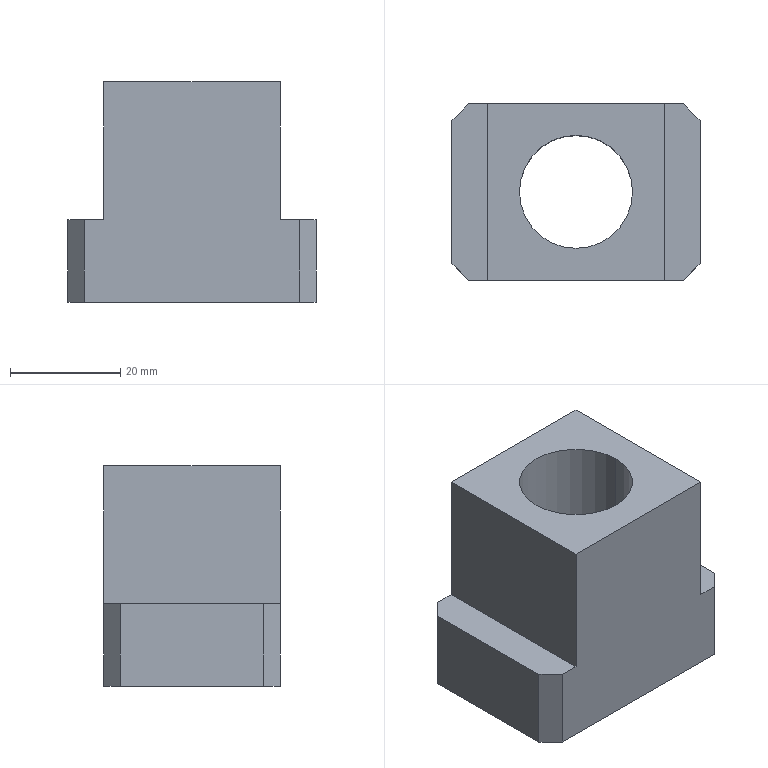Part | SolidWorks | features BaseBody 1 | 1 solid | 16 faces | box 45 x 32 x 40 mm | volume 33727 mm3 | plane 14 | cylinder 2 | commonest cylinder face diameters 20.5 x2
STEP:
#1=CARTESIAN_POINT('',(-10.25,0.,-27.5));
#2=VERTEX_POINT('',#1);
#3=CARTESIAN_POINT('',(10.25,0.,-27.5));
#4=VERTEX_POINT('',#3);
#5=CARTESIAN_POINT('',(0.,0.,-27.5));
#6=DIRECTION('',(0.,0.,1.));
#7=DIRECTION('',(1.,0.,0.));
#8=AXIS2_PLACEMENT_3D('',#5,#6,#7);
#9=CIRCLE('',#8,10.25);
#10=EDGE_CURVE('',#2,#4,#9,.T.);
#11=ORIENTED_EDGE('',*,*,#10,.F.);
#12=CARTESIAN_POINT('',(-10.25,0.,12.5));
#13=VERTEX_POINT('',#12);
#14=CARTESIAN_POINT('',(-10.25,0.,12.5));
#15=DIRECTION('',(0.,0.,1.));
#16=VECTOR('',#15,1000.);
#17=LINE('',#14,#16);
#18=EDGE_CURVE('',#2,#13,#17,.T.);
#19=ORIENTED_EDGE('',*,*,#18,.T.);
#20=CARTESIAN_POINT('',(10.25,0.,12.5));
#21=VERTEX_POINT('',#20);
#22=CARTESIAN_POINT('',(0.,0.,12.5));
#23=DIRECTION('',(0.,0.,1.));
#24=DIRECTION('',(1.,0.,0.));
#25=AXIS2_PLACEMENT_3D('',#22,#23,#24);
#26=CIRCLE('',#25,10.25);
#27=EDGE_CURVE('',#13,#21,#26,.T.);
#28=ORIENTED_EDGE('',*,*,#27,.T.);
#29=CARTESIAN_POINT('',(10.25,0.,12.5));
#30=DIRECTION('',(0.,0.,1.));
#31=VECTOR('',#30,1000.);
#32=LINE('',#29,#31);
#33=EDGE_CURVE('',#4,#21,#32,.T.);
#34=ORIENTED_EDGE('',*,*,#33,.F.);
#35=EDGE_LOOP('',(#11,#19,#28,#34));
#36=FACE_OUTER_BOUND('',#35,.T.);
#37=CARTESIAN_POINT('',(0.,0.,12.5));
#38=DIRECTION('',(0.,0.,1.));
#39=DIRECTION('',(1.,0.,0.));
#40=AXIS2_PLACEMENT_3D('',#37,#38,#39);
#41=CYLINDRICAL_SURFACE('',#40,10.25);
#42=ADVANCED_FACE('',(#36),#41,.F.);
#43=CARTESIAN_POINT('',(-16.,16.,-12.5));
#44=VERTEX_POINT('',#43);
#45=CARTESIAN_POINT('',(-16.,-16.,-12.5));
#46=VERTEX_POINT('',#45);
#47=CARTESIAN_POINT('',(-16.,16.,-12.5));
#48=DIRECTION('',(0.,-1.,0.));
#49=VECTOR('',#48,1000.);
#50=LINE('',#47,#49);
#51=EDGE_CURVE('',#44,#46,#50,.T.);
#52=ORIENTED_EDGE('',*,*,#51,.T.);
#53=CARTESIAN_POINT('',(-16.,-16.,12.5));
#54=VERTEX_POINT('',#53);
#55=CARTESIAN_POINT('',(-16.,-16.,12.5));
#56=DIRECTION('',(0.,0.,-1.));
#57=VECTOR('',#56,1000.);
#58=LINE('',#55,#57);
#59=EDGE_CURVE('',#54,#46,#58,.T.);
#60=ORIENTED_EDGE('',*,*,#59,.F.);
#61=CARTESIAN_POINT('',(-16.,16.,12.5));
#62=VERTEX_POINT('',#61);
#63=CARTESIAN_POINT('',(-16.,16.,12.5));
#64=DIRECTION('',(0.,-1.,0.));
#65=VECTOR('',#64,1000.);
#66=LINE('',#63,#65);
#67=EDGE_CURVE('',#62,#54,#66,.T.);
#68=ORIENTED_EDGE('',*,*,#67,.F.);
#69=CARTESIAN_POINT('',(-16.,16.,12.5));
#70=DIRECTION('',(0.,0.,-1.));
#71=VECTOR('',#70,1000.);
#72=LINE('',#69,#71);
#73=EDGE_CURVE('',#62,#44,#72,.T.);
#74=ORIENTED_EDGE('',*,*,#73,.T.);
#75=EDGE_LOOP('',(#52,#60,#68,#74));
#76=FACE_OUTER_BOUND('',#75,.T.);
#77=CARTESIAN_POINT('',(-16.,16.,12.5));
#78=DIRECTION('',(1.,0.,0.));
#79=DIRECTION('',(0.,1.,0.));
#80=AXIS2_PLACEMENT_3D('',#77,#78,#79);
#81=PLANE('',#80);
#82=ADVANCED_FACE('',(#76),#81,.F.);
#83=CARTESIAN_POINT('',(19.5,-16.,-27.5));
#84=VERTEX_POINT('',#83);
#85=CARTESIAN_POINT('',(-19.5,-16.,-27.5));
#86=VERTEX_POINT('',#85);
#87=CARTESIAN_POINT('',(-22.5,-16.,-27.5));
#88=DIRECTION('',(-1.,0.,0.));
#89=VECTOR('',#88,1000.);
#90=LINE('',#87,#89);
#91=EDGE_CURVE('',#84,#86,#90,.T.);
#92=ORIENTED_EDGE('',*,*,#91,.F.);
#93=CARTESIAN_POINT('',(19.5,-16.,-12.5));
#94=VERTEX_POINT('',#93);
#95=CARTESIAN_POINT('',(19.5,-16.,12.5));
#96=DIRECTION('',(0.,0.,1.));
#97=VECTOR('',#96,1000.);
#98=LINE('',#95,#97);
#99=EDGE_CURVE('',#84,#94,#98,.T.);
#100=ORIENTED_EDGE('',*,*,#99,.T.);
#101=CARTESIAN_POINT('',(16.,-16.,-12.5));
#102=VERTEX_POINT('',#101);
#103=CARTESIAN_POINT('',(-22.5,-16.,-12.5));
#104=DIRECTION('',(-1.,0.,0.));
#105=VECTOR('',#104,1000.);
#106=LINE('',#103,#105);
#107=EDGE_CURVE('',#94,#102,#106,.T.);
#108=ORIENTED_EDGE('',*,*,#107,.T.);
#109=CARTESIAN_POINT('',(16.,-16.,12.5));
#110=VERTEX_POINT('',#109);
#111=CARTESIAN_POINT('',(16.,-16.,12.5));
#112=DIRECTION('',(0.,0.,-1.));
#113=VECTOR('',#112,1000.);
#114=LINE('',#111,#113);
#115=EDGE_CURVE('',#110,#102,#114,.T.);
#116=ORIENTED_EDGE('',*,*,#115,.F.);
#117=CARTESIAN_POINT('',(16.,-16.,12.5));
#118=DIRECTION('',(1.,0.,0.));
#119=VECTOR('',#118,1000.);
#120=LINE('',#117,#119);
#121=EDGE_CURVE('',#54,#110,#120,.T.);
#122=ORIENTED_EDGE('',*,*,#121,.F.);
#123=ORIENTED_EDGE('',*,*,#59,.T.);
#124=CARTESIAN_POINT('',(-19.5,-16.,-12.5));
#125=VERTEX_POINT('',#124);
#126=CARTESIAN_POINT('',(-22.5,-16.,-12.5));
#127=DIRECTION('',(-1.,0.,0.));
#128=VECTOR('',#127,1000.);
#129=LINE('',#126,#128);
#130=EDGE_CURVE('',#46,#125,#129,.T.);
#131=ORIENTED_EDGE('',*,*,#130,.T.);
#132=CARTESIAN_POINT('',(-19.5,-16.,12.5));
#133=DIRECTION('',(0.,0.,-1.));
#134=VECTOR('',#133,1000.);
#135=LINE('',#132,#134);
#136=EDGE_CURVE('',#125,#86,#135,.T.);
#137=ORIENTED_EDGE('',*,*,#136,.T.);
#138=EDGE_LOOP('',(#92,#100,#108,#116,#122,#123,#131,#137));
#139=FACE_OUTER_BOUND('',#138,.T.);
#140=CARTESIAN_POINT('',(16.,-16.,12.5));
#141=DIRECTION('',(0.,1.,0.));
#142=DIRECTION('',(-1.,0.,0.));
#143=AXIS2_PLACEMENT_3D('',#140,#141,#142);
#144=PLANE('',#143);
#145=ADVANCED_FACE('',(#139),#144,.F.);
#146=CARTESIAN_POINT('',(16.,16.,-12.5));
#147=VERTEX_POINT('',#146);
#148=CARTESIAN_POINT('',(16.,16.,-12.5));
#149=DIRECTION('',(0.,1.,0.));
#150=VECTOR('',#149,1000.);
#151=LINE('',#148,#150);
#152=EDGE_CURVE('',#102,#147,#151,.T.);
#153=ORIENTED_EDGE('',*,*,#152,.T.);
#154=CARTESIAN_POINT('',(16.,16.,12.5));
#155=VERTEX_POINT('',#154);
#156=CARTESIAN_POINT('',(16.,16.,12.5));
#157=DIRECTION('',(0.,0.,-1.));
#158=VECTOR('',#157,1000.);
#159=LINE('',#156,#158);
#160=EDGE_CURVE('',#155,#147,#159,.T.);
#161=ORIENTED_EDGE('',*,*,#160,.F.);
#162=CARTESIAN_POINT('',(16.,16.,12.5));
#163=DIRECTION('',(0.,1.,0.));
#164=VECTOR('',#163,1000.);
#165=LINE('',#162,#164);
#166=EDGE_CURVE('',#110,#155,#165,.T.);
#167=ORIENTED_EDGE('',*,*,#166,.F.);
#168=ORIENTED_EDGE('',*,*,#115,.T.);
#169=EDGE_LOOP('',(#153,#161,#167,#168));
#170=FACE_OUTER_BOUND('',#169,.T.);
#171=CARTESIAN_POINT('',(16.,16.,12.5));
#172=DIRECTION('',(-1.,0.,0.));
#173=DIRECTION('',(0.,-1.,0.));
#174=AXIS2_PLACEMENT_3D('',#171,#172,#173);
#175=PLANE('',#174);
#176=ADVANCED_FACE('',(#170),#175,.F.);
#177=CARTESIAN_POINT('',(19.5,16.,-12.5));
#178=VERTEX_POINT('',#177);
#179=CARTESIAN_POINT('',(-22.5,16.,-12.5));
#180=DIRECTION('',(1.,0.,0.));
#181=VECTOR('',#180,1000.);
#182=LINE('',#179,#181);
#183=EDGE_CURVE('',#147,#178,#182,.T.);
#184=ORIENTED_EDGE('',*,*,#183,.T.);
#185=CARTESIAN_POINT('',(19.5,16.,-27.5));
#186=VERTEX_POINT('',#185);
#187=CARTESIAN_POINT('',(19.5,16.,12.5));
#188=DIRECTION('',(0.,0.,-1.));
#189=VECTOR('',#188,1000.);
#190=LINE('',#187,#189);
#191=EDGE_CURVE('',#178,#186,#190,.T.);
#192=ORIENTED_EDGE('',*,*,#191,.T.);
#193=CARTESIAN_POINT('',(-19.5,16.,-27.5));
#194=VERTEX_POINT('',#193);
#195=CARTESIAN_POINT('',(-22.5,16.,-27.5));
#196=DIRECTION('',(1.,0.,0.));
#197=VECTOR('',#196,1000.);
#198=LINE('',#195,#197);
#199=EDGE_CURVE('',#194,#186,#198,.T.);
#200=ORIENTED_EDGE('',*,*,#199,.F.);
#201=CARTESIAN_POINT('',(-19.5,16.,-12.5));
#202=VERTEX_POINT('',#201);
#203=CARTESIAN_POINT('',(-19.5,16.,12.5));
#204=DIRECTION('',(0.,0.,1.));
#205=VECTOR('',#204,1000.);
#206=LINE('',#203,#205);
#207=EDGE_CURVE('',#194,#202,#206,.T.);
#208=ORIENTED_EDGE('',*,*,#207,.T.);
#209=CARTESIAN_POINT('',(-22.5,16.,-12.5));
#210=DIRECTION('',(1.,0.,0.));
#211=VECTOR('',#210,1000.);
#212=LINE('',#209,#211);
#213=EDGE_CURVE('',#202,#44,#212,.T.);
#214=ORIENTED_EDGE('',*,*,#213,.T.);
#215=ORIENTED_EDGE('',*,*,#73,.F.);
#216=CARTESIAN_POINT('',(16.,16.,12.5));
#217=DIRECTION('',(-1.,0.,0.));
#218=VECTOR('',#217,1000.);
#219=LINE('',#216,#218);
#220=EDGE_CURVE('',#155,#62,#219,.T.);
#221=ORIENTED_EDGE('',*,*,#220,.F.);
#222=ORIENTED_EDGE('',*,*,#160,.T.);
#223=EDGE_LOOP('',(#184,#192,#200,#208,#214,#215,#221,#222));
#224=FACE_OUTER_BOUND('',#223,.T.);
#225=CARTESIAN_POINT('',(16.,16.,12.5));
#226=DIRECTION('',(0.,-1.,0.));
#227=DIRECTION('',(1.,0.,0.));
#228=AXIS2_PLACEMENT_3D('',#225,#226,#227);
#229=PLANE('',#228);
#230=ADVANCED_FACE('',(#224),#229,.F.);
#231=CARTESIAN_POINT('',(0.,0.,12.5));
#232=DIRECTION('',(0.,0.,1.));
#233=DIRECTION('',(1.,0.,0.));
#234=AXIS2_PLACEMENT_3D('',#231,#232,#233);
#235=CIRCLE('',#234,10.25);
#236=EDGE_CURVE('',#21,#13,#235,.T.);
#237=ORIENTED_EDGE('',*,*,#236,.F.);
#238=ORIENTED_EDGE('',*,*,#27,.F.);
#239=EDGE_LOOP('',(#237,#238));
#240=FACE_BOUND('',#239,.T.);
#241=ORIENTED_EDGE('',*,*,#67,.T.);
#242=ORIENTED_EDGE('',*,*,#121,.T.);
#243=ORIENTED_EDGE('',*,*,#166,.T.);
#244=ORIENTED_EDGE('',*,*,#220,.T.);
#245=EDGE_LOOP('',(#241,#242,#243,#244));
#246=FACE_OUTER_BOUND('',#245,.T.);
#247=CARTESIAN_POINT('',(-16.,-16.,12.5));
#248=DIRECTION('',(0.,0.,-1.));
#249=DIRECTION('',(-1.,0.,0.));
#250=AXIS2_PLACEMENT_3D('',#247,#248,#249);
#251=PLANE('',#250);
#252=ADVANCED_FACE('',(#240,#246),#251,.F.);
#253=CARTESIAN_POINT('',(-22.5,-13.,-12.5));
#254=VERTEX_POINT('',#253);
#255=CARTESIAN_POINT('',(-22.5,13.,-12.5));
#256=VERTEX_POINT('',#255);
#257=CARTESIAN_POINT('',(-22.5,16.,-12.5));
#258=DIRECTION('',(0.,1.,0.));
#259=VECTOR('',#258,1000.);
#260=LINE('',#257,#259);
#261=EDGE_CURVE('',#254,#256,#260,.T.);
#262=ORIENTED_EDGE('',*,*,#261,.F.);
#263=CARTESIAN_POINT('',(1.5,-37.,-12.5));
#264=DIRECTION('',(0.7071,-0.7071,0.));
#265=VECTOR('',#264,1000.);
#266=LINE('',#263,#265);
#267=EDGE_CURVE('',#254,#125,#266,.T.);
#268=ORIENTED_EDGE('',*,*,#267,.T.);
#269=ORIENTED_EDGE('',*,*,#130,.F.);
#270=ORIENTED_EDGE('',*,*,#51,.F.);
#271=ORIENTED_EDGE('',*,*,#213,.F.);
#272=CARTESIAN_POINT('',(-14.5,21.,-12.5));
#273=DIRECTION('',(-0.7071,-0.7071,0.));
#274=VECTOR('',#273,1000.);
#275=LINE('',#272,#274);
#276=EDGE_CURVE('',#202,#256,#275,.T.);
#277=ORIENTED_EDGE('',*,*,#276,.T.);
#278=EDGE_LOOP('',(#262,#268,#269,#270,#271,#277));
#279=FACE_OUTER_BOUND('',#278,.T.);
#280=CARTESIAN_POINT('',(22.5,-16.,-12.5));
#281=DIRECTION('',(0.,0.,1.));
#282=DIRECTION('',(1.,0.,0.));
#283=AXIS2_PLACEMENT_3D('',#280,#281,#282);
#284=PLANE('',#283);
#285=ADVANCED_FACE('',(#279),#284,.T.);
#286=CARTESIAN_POINT('',(22.5,13.,-12.5));
#287=VERTEX_POINT('',#286);
#288=CARTESIAN_POINT('',(22.5,-13.,-12.5));
#289=VERTEX_POINT('',#288);
#290=CARTESIAN_POINT('',(22.5,16.,-12.5));
#291=DIRECTION('',(0.,-1.,0.));
#292=VECTOR('',#291,1000.);
#293=LINE('',#290,#292);
#294=EDGE_CURVE('',#287,#289,#293,.T.);
#295=ORIENTED_EDGE('',*,*,#294,.F.);
#296=CARTESIAN_POINT('',(37.,-1.5,-12.5));
#297=DIRECTION('',(-0.7071,0.7071,0.));
#298=VECTOR('',#297,1000.);
#299=LINE('',#296,#298);
#300=EDGE_CURVE('',#287,#178,#299,.T.);
#301=ORIENTED_EDGE('',*,*,#300,.T.);
#302=ORIENTED_EDGE('',*,*,#183,.F.);
#303=ORIENTED_EDGE('',*,*,#152,.F.);
#304=ORIENTED_EDGE('',*,*,#107,.F.);
#305=CARTESIAN_POINT('',(21.,-14.5,-12.5));
#306=DIRECTION('',(0.7071,0.7071,0.));
#307=VECTOR('',#306,1000.);
#308=LINE('',#305,#307);
#309=EDGE_CURVE('',#94,#289,#308,.T.);
#310=ORIENTED_EDGE('',*,*,#309,.T.);
#311=EDGE_LOOP('',(#295,#301,#302,#303,#304,#310));
#312=FACE_OUTER_BOUND('',#311,.T.);
#313=CARTESIAN_POINT('',(22.5,-16.,-12.5));
#314=DIRECTION('',(0.,0.,1.));
#315=DIRECTION('',(1.,0.,0.));
#316=AXIS2_PLACEMENT_3D('',#313,#314,#315);
#317=PLANE('',#316);
#318=ADVANCED_FACE('',(#312),#317,.T.);
#319=CARTESIAN_POINT('',(22.5,13.,-27.5));
#320=VERTEX_POINT('',#319);
#321=CARTESIAN_POINT('',(22.5,-13.,-27.5));
#322=VERTEX_POINT('',#321);
#323=CARTESIAN_POINT('',(22.5,16.,-27.5));
#324=DIRECTION('',(0.,-1.,0.));
#325=VECTOR('',#324,1000.);
#326=LINE('',#323,#325);
#327=EDGE_CURVE('',#320,#322,#326,.T.);
#328=ORIENTED_EDGE('',*,*,#327,.F.);
#329=CARTESIAN_POINT('',(22.5,13.,-27.5));
#330=DIRECTION('',(0.,0.,1.));
#331=VECTOR('',#330,1000.);
#332=LINE('',#329,#331);
#333=EDGE_CURVE('',#320,#287,#332,.T.);
#334=ORIENTED_EDGE('',*,*,#333,.T.);
#335=ORIENTED_EDGE('',*,*,#294,.T.);
#336=CARTESIAN_POINT('',(22.5,-13.,-27.5));
#337=DIRECTION('',(0.,0.,-1.));
#338=VECTOR('',#337,1000.);
#339=LINE('',#336,#338);
#340=EDGE_CURVE('',#289,#322,#339,.T.);
#341=ORIENTED_EDGE('',*,*,#340,.T.);
#342=EDGE_LOOP('',(#328,#334,#335,#341));
#343=FACE_OUTER_BOUND('',#342,.T.);
#344=CARTESIAN_POINT('',(22.5,16.,-27.5));
#345=DIRECTION('',(-1.,0.,0.));
#346=DIRECTION('',(0.,-1.,0.));
#347=AXIS2_PLACEMENT_3D('',#344,#345,#346);
#348=PLANE('',#347);
#349=ADVANCED_FACE('',(#343),#348,.F.);
#350=CARTESIAN_POINT('',(-22.5,-13.,-27.5));
#351=VERTEX_POINT('',#350);
#352=CARTESIAN_POINT('',(-22.5,13.,-27.5));
#353=VERTEX_POINT('',#352);
#354=CARTESIAN_POINT('',(-22.5,16.,-27.5));
#355=DIRECTION('',(0.,1.,0.));
#356=VECTOR('',#355,1000.);
#357=LINE('',#354,#356);
#358=EDGE_CURVE('',#351,#353,#357,.T.);
#359=ORIENTED_EDGE('',*,*,#358,.F.);
#360=CARTESIAN_POINT('',(-22.5,-13.,-27.5));
#361=DIRECTION('',(0.,0.,1.));
#362=VECTOR('',#361,1000.);
#363=LINE('',#360,#362);
#364=EDGE_CURVE('',#351,#254,#363,.T.);
#365=ORIENTED_EDGE('',*,*,#364,.T.);
#366=ORIENTED_EDGE('',*,*,#261,.T.);
#367=CARTESIAN_POINT('',(-22.5,13.,-27.5));
#368=DIRECTION('',(0.,0.,-1.));
#369=VECTOR('',#368,1000.);
#370=LINE('',#367,#369);
#371=EDGE_CURVE('',#256,#353,#370,.T.);
#372=ORIENTED_EDGE('',*,*,#371,.T.);
#373=EDGE_LOOP('',(#359,#365,#366,#372));
#374=FACE_OUTER_BOUND('',#373,.T.);
#375=CARTESIAN_POINT('',(-22.5,16.,-27.5));
#376=DIRECTION('',(1.,0.,0.));
#377=DIRECTION('',(0.,0.,-1.));
#378=AXIS2_PLACEMENT_3D('',#375,#376,#377);
#379=PLANE('',#378);
#380=ADVANCED_FACE('',(#374),#379,.F.);
#381=CARTESIAN_POINT('',(0.,0.,-27.5));
#382=DIRECTION('',(0.,0.,1.));
#383=DIRECTION('',(1.,0.,0.));
#384=AXIS2_PLACEMENT_3D('',#381,#382,#383);
#385=CIRCLE('',#384,10.25);
#386=EDGE_CURVE('',#4,#2,#385,.T.);
#387=ORIENTED_EDGE('',*,*,#386,.T.);
#388=ORIENTED_EDGE('',*,*,#10,.T.);
#389=EDGE_LOOP('',(#387,#388));
#390=FACE_BOUND('',#389,.T.);
#391=ORIENTED_EDGE('',*,*,#199,.T.);
#392=CARTESIAN_POINT('',(22.5,13.,-27.5));
#393=DIRECTION('',(0.7071,-0.7071,0.));
#394=VECTOR('',#393,1000.);
#395=LINE('',#392,#394);
#396=EDGE_CURVE('',#186,#320,#395,.T.);
#397=ORIENTED_EDGE('',*,*,#396,.T.);
#398=ORIENTED_EDGE('',*,*,#327,.T.);
#399=CARTESIAN_POINT('',(19.5,-16.,-27.5));
#400=DIRECTION('',(-0.7071,-0.7071,0.));
#401=VECTOR('',#400,1000.);
#402=LINE('',#399,#401);
#403=EDGE_CURVE('',#322,#84,#402,.T.);
#404=ORIENTED_EDGE('',*,*,#403,.T.);
#405=ORIENTED_EDGE('',*,*,#91,.T.);
#406=CARTESIAN_POINT('',(-22.5,-13.,-27.5));
#407=DIRECTION('',(-0.7071,0.7071,0.));
#408=VECTOR('',#407,1000.);
#409=LINE('',#406,#408);
#410=EDGE_CURVE('',#86,#351,#409,.T.);
#411=ORIENTED_EDGE('',*,*,#410,.T.);
#412=ORIENTED_EDGE('',*,*,#358,.T.);
#413=CARTESIAN_POINT('',(-19.5,16.,-27.5));
#414=DIRECTION('',(0.7071,0.7071,0.));
#415=VECTOR('',#414,1000.);
#416=LINE('',#413,#415);
#417=EDGE_CURVE('',#353,#194,#416,.T.);
#418=ORIENTED_EDGE('',*,*,#417,.T.);
#419=EDGE_LOOP('',(#391,#397,#398,#404,#405,#411,#412,#418));
#420=FACE_OUTER_BOUND('',#419,.T.);
#421=CARTESIAN_POINT('',(22.5,-16.,-27.5));
#422=DIRECTION('',(0.,0.,1.));
#423=DIRECTION('',(1.,0.,0.));
#424=AXIS2_PLACEMENT_3D('',#421,#422,#423);
#425=PLANE('',#424);
#426=ADVANCED_FACE('',(#390,#420),#425,.F.);
#427=ORIENTED_EDGE('',*,*,#18,.F.);
#428=ORIENTED_EDGE('',*,*,#386,.F.);
#429=ORIENTED_EDGE('',*,*,#33,.T.);
#430=ORIENTED_EDGE('',*,*,#236,.T.);
#431=EDGE_LOOP('',(#427,#428,#429,#430));
#432=FACE_OUTER_BOUND('',#431,.T.);
#433=CARTESIAN_POINT('',(0.,0.,12.5));
#434=DIRECTION('',(0.,0.,1.));
#435=DIRECTION('',(1.,0.,0.));
#436=AXIS2_PLACEMENT_3D('',#433,#434,#435);
#437=CYLINDRICAL_SURFACE('',#436,10.25);
#438=ADVANCED_FACE('',(#432),#437,.F.);
#439=ORIENTED_EDGE('',*,*,#396,.F.);
#440=ORIENTED_EDGE('',*,*,#191,.F.);
#441=ORIENTED_EDGE('',*,*,#300,.F.);
#442=ORIENTED_EDGE('',*,*,#333,.F.);
#443=EDGE_LOOP('',(#439,#440,#441,#442));
#444=FACE_OUTER_BOUND('',#443,.T.);
#445=CARTESIAN_POINT('',(22.5,13.,-27.5));
#446=DIRECTION('',(-0.7071,-0.7071,0.));
#447=DIRECTION('',(0.7071,-0.7071,0.));
#448=AXIS2_PLACEMENT_3D('',#445,#446,#447);
#449=PLANE('',#448);
#450=ADVANCED_FACE('',(#444),#449,.F.);
#451=ORIENTED_EDGE('',*,*,#403,.F.);
#452=ORIENTED_EDGE('',*,*,#340,.F.);
#453=ORIENTED_EDGE('',*,*,#309,.F.);
#454=ORIENTED_EDGE('',*,*,#99,.F.);
#455=EDGE_LOOP('',(#451,#452,#453,#454));
#456=FACE_OUTER_BOUND('',#455,.T.);
#457=CARTESIAN_POINT('',(19.5,-16.,12.5));
#458=DIRECTION('',(-0.7071,0.7071,0.));
#459=DIRECTION('',(-0.7071,-0.7071,0.));
#460=AXIS2_PLACEMENT_3D('',#457,#458,#459);
#461=PLANE('',#460);
#462=ADVANCED_FACE('',(#456),#461,.F.);
#463=ORIENTED_EDGE('',*,*,#410,.F.);
#464=ORIENTED_EDGE('',*,*,#136,.F.);
#465=ORIENTED_EDGE('',*,*,#267,.F.);
#466=ORIENTED_EDGE('',*,*,#364,.F.);
#467=EDGE_LOOP('',(#463,#464,#465,#466));
#468=FACE_OUTER_BOUND('',#467,.T.);
#469=CARTESIAN_POINT('',(-22.5,-13.,-27.5));
#470=DIRECTION('',(0.7071,0.7071,0.));
#471=DIRECTION('',(-0.7071,0.7071,0.));
#472=AXIS2_PLACEMENT_3D('',#469,#470,#471);
#473=PLANE('',#472);
#474=ADVANCED_FACE('',(#468),#473,.F.);
#475=ORIENTED_EDGE('',*,*,#417,.F.);
#476=ORIENTED_EDGE('',*,*,#371,.F.);
#477=ORIENTED_EDGE('',*,*,#276,.F.);
#478=ORIENTED_EDGE('',*,*,#207,.F.);
#479=EDGE_LOOP('',(#475,#476,#477,#478));
#480=FACE_OUTER_BOUND('',#479,.T.);
#481=CARTESIAN_POINT('',(-19.5,16.,12.5));
#482=DIRECTION('',(0.7071,-0.7071,0.));
#483=DIRECTION('',(0.7071,0.7071,0.));
#484=AXIS2_PLACEMENT_3D('',#481,#482,#483);
#485=PLANE('',#484);
#486=ADVANCED_FACE('',(#480),#485,.F.);
#487=CLOSED_SHELL('',(#42,#82,#145,#176,#230,#252,#285,#318,#349,#380,#426,#438,#450,#462,#474,#486));
#488=MANIFOLD_SOLID_BREP('',#487);
#489=CARTESIAN_POINT('',(0.,0.,0.));
#490=DIRECTION('',(0.,0.,1.));
#491=DIRECTION('',(1.,0.,0.));
#492=AXIS2_PLACEMENT_3D('',#489,#490,#491);
#493=(LENGTH_UNIT()NAMED_UNIT(*)SI_UNIT(.MILLI.,.METRE.));
#494=UNCERTAINTY_MEASURE_WITH_UNIT(LENGTH_MEASURE(0.00001),#493,'','');
#495=(NAMED_UNIT(*)PLANE_ANGLE_UNIT()SI_UNIT($,.RADIAN.));
#496=(NAMED_UNIT(*)SI_UNIT($,.STERADIAN.)SOLID_ANGLE_UNIT());
#497=(GEOMETRIC_REPRESENTATION_CONTEXT(3)GLOBAL_UNCERTAINTY_ASSIGNED_CONTEXT((#494))GLOBAL_UNIT_ASSIGNED_CONTEXT((#493,#495,#496))REPRESENTATION_CONTEXT('',''));
#498=ADVANCED_BREP_SHAPE_REPRESENTATION('',(#488,#492),#497);